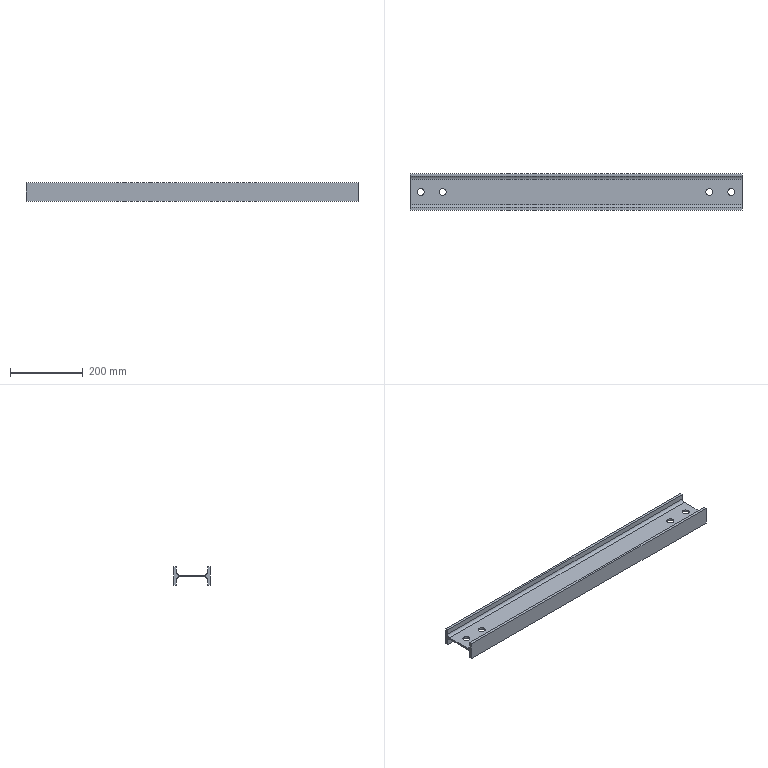Part | STEP file | 粉仓辅梁15主体_Default<As Machined> | 1 solid | 26 faces | box 915 x 100 x 50 mm | volume 1078548 mm3 | plane 14 | cylinder 12 | commonest cylinder face diameters 19 x8 16 x4